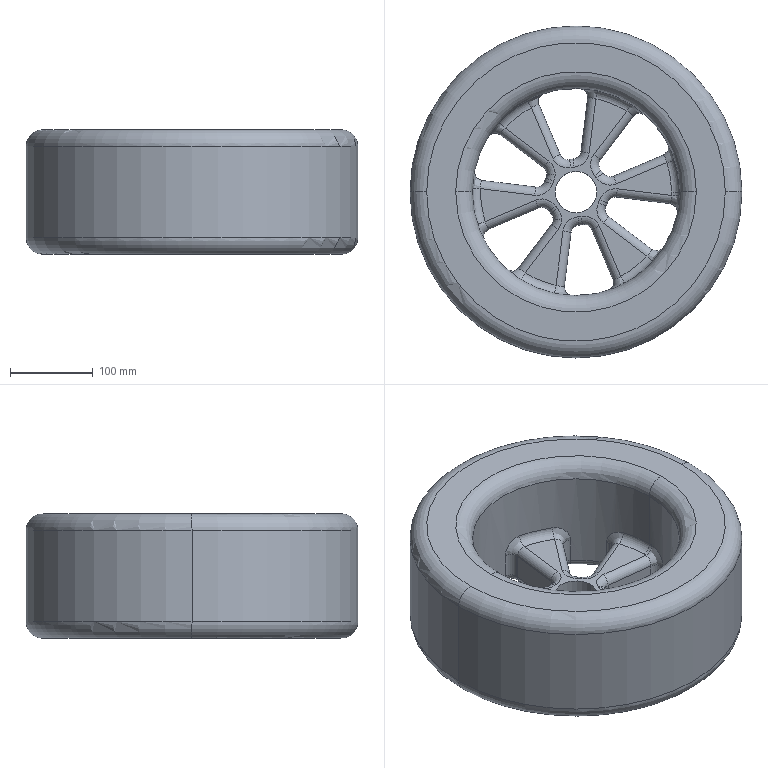Part | SolidWorks | features Fillet 2, ICE 2, CirPattern 1, Extrusion 1 | 1 solid | 168 faces | box 400 x 400 x 150 mm | volume 12435033 mm3 | torus 75 | cylinder 66 | plane 15 | spline 12 | commonest cylinder face diameters 20 x54 80 x6 50 x2 250 x2 400 x2